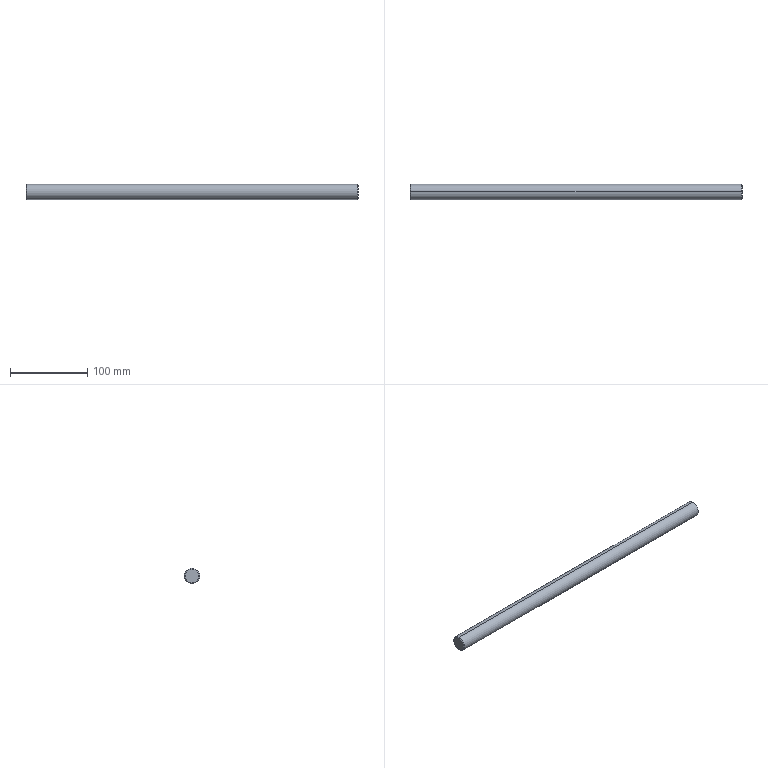Part | STEP file | 001-006-SAD21_D20_L430 | 1 solid | 8 faces | box 430 x 20 x 20 mm | volume 135028 mm3 | cone 4 | cylinder 2 | plane 2 | commonest cylinder face diameters 20 x2
STEP:
#1=CARTESIAN_POINT('',(0.,0.,0.));
#2=DIRECTION('',(0.,0.,1.));
#3=DIRECTION('',(1.,0.,0.));
#4=AXIS2_PLACEMENT_3D('',#1,#2,#3);
#5=CARTESIAN_POINT('',(430.,0.,9.));
#6=VERTEX_POINT('',#5);
#7=CARTESIAN_POINT('',(430.,0.,-9.));
#8=VERTEX_POINT('',#7);
#9=CARTESIAN_POINT('',(430.,0.,0.));
#10=DIRECTION('',(-1.,0.,0.));
#11=DIRECTION('',(0.,0.,1.));
#12=AXIS2_PLACEMENT_3D('',#9,#10,#11);
#13=CIRCLE('',#12,9.);
#14=CARTESIAN_POINT('',(430.,0.,0.));
#15=DIRECTION('',(-1.,0.,0.));
#16=DIRECTION('',(0.,0.,1.));
#17=AXIS2_PLACEMENT_3D('',#14,#15,#16);
#18=CONICAL_SURFACE('',#17,9.,0.7854);
#19=CARTESIAN_POINT('',(0.,0.));
#20=DIRECTION('',(1.,0.));
#21=VECTOR('',#20,1.);
#22=LINE('',#19,#21);
#23=(GEOMETRIC_REPRESENTATION_CONTEXT(2)PARAMETRIC_REPRESENTATION_CONTEXT()REPRESENTATION_CONTEXT('',''));
#24=DEFINITIONAL_REPRESENTATION('',(#22),#23);
#25=PCURVE('',#18,#24);
#26=CARTESIAN_POINT('',(430.,9.,0.));
#27=DIRECTION('',(-1.,0.,0.));
#28=DIRECTION('',(0.,0.,1.));
#29=AXIS2_PLACEMENT_3D('',#26,#27,#28);
#30=PLANE('',#29);
#31=CARTESIAN_POINT('',(0.,-9.));
#32=DIRECTION('',(1.,0.));
#33=AXIS2_PLACEMENT_2D('',#31,#32);
#34=CIRCLE('',#33,9.);
#35=(GEOMETRIC_REPRESENTATION_CONTEXT(2)PARAMETRIC_REPRESENTATION_CONTEXT()REPRESENTATION_CONTEXT('',''));
#36=DEFINITIONAL_REPRESENTATION('',(#34),#35);
#37=PCURVE('',#30,#36);
#38=SURFACE_CURVE('',#13,(#25,#37),.PCURVE_S1.);
#39=EDGE_CURVE('',#6,#8,#38,.T.);
#40=ORIENTED_EDGE('',*,*,#39,.T.);
#41=CARTESIAN_POINT('',(429.,0.,-10.));
#42=VERTEX_POINT('',#41);
#43=CARTESIAN_POINT('',(430.,0.,-9.));
#44=DIRECTION('',(-0.7071,0.,-0.7071));
#45=VECTOR('',#44,1.);
#46=LINE('',#43,#45);
#47=CARTESIAN_POINT('',(3.142,0.));
#48=DIRECTION('',(0.,1.));
#49=VECTOR('',#48,1.);
#50=LINE('',#47,#49);
#51=(GEOMETRIC_REPRESENTATION_CONTEXT(2)PARAMETRIC_REPRESENTATION_CONTEXT()REPRESENTATION_CONTEXT('',''));
#52=DEFINITIONAL_REPRESENTATION('',(#50),#51);
#53=PCURVE('',#18,#52);
#54=CARTESIAN_POINT('',(430.,0.,0.));
#55=DIRECTION('',(-1.,0.,0.));
#56=DIRECTION('',(0.,0.,1.));
#57=AXIS2_PLACEMENT_3D('',#54,#55,#56);
#58=CONICAL_SURFACE('',#57,9.,0.7854);
#59=CARTESIAN_POINT('',(3.142,0.));
#60=DIRECTION('',(0.,1.));
#61=VECTOR('',#60,1.);
#62=LINE('',#59,#61);
#63=(GEOMETRIC_REPRESENTATION_CONTEXT(2)PARAMETRIC_REPRESENTATION_CONTEXT()REPRESENTATION_CONTEXT('',''));
#64=DEFINITIONAL_REPRESENTATION('',(#62),#63);
#65=PCURVE('',#58,#64);
#66=SURFACE_CURVE('',#46,(#53,#65),.PCURVE_S1.);
#67=EDGE_CURVE('',#8,#42,#66,.T.);
#68=ORIENTED_EDGE('',*,*,#67,.T.);
#69=CARTESIAN_POINT('',(429.,0.,10.));
#70=VERTEX_POINT('',#69);
#71=CARTESIAN_POINT('',(429.,0.,0.));
#72=DIRECTION('',(-1.,0.,0.));
#73=DIRECTION('',(0.,0.,1.));
#74=AXIS2_PLACEMENT_3D('',#71,#72,#73);
#75=CIRCLE('',#74,10.);
#76=CARTESIAN_POINT('',(0.,1.));
#77=DIRECTION('',(1.,0.));
#78=VECTOR('',#77,1.);
#79=LINE('',#76,#78);
#80=(GEOMETRIC_REPRESENTATION_CONTEXT(2)PARAMETRIC_REPRESENTATION_CONTEXT()REPRESENTATION_CONTEXT('',''));
#81=DEFINITIONAL_REPRESENTATION('',(#79),#80);
#82=PCURVE('',#18,#81);
#83=CARTESIAN_POINT('',(430.,0.,0.));
#84=DIRECTION('',(-1.,0.,0.));
#85=DIRECTION('',(0.,0.,1.));
#86=AXIS2_PLACEMENT_3D('',#83,#84,#85);
#87=CYLINDRICAL_SURFACE('',#86,10.);
#88=CARTESIAN_POINT('',(0.,1.));
#89=DIRECTION('',(1.,0.));
#90=VECTOR('',#89,1.);
#91=LINE('',#88,#90);
#92=(GEOMETRIC_REPRESENTATION_CONTEXT(2)PARAMETRIC_REPRESENTATION_CONTEXT()REPRESENTATION_CONTEXT('',''));
#93=DEFINITIONAL_REPRESENTATION('',(#91),#92);
#94=PCURVE('',#87,#93);
#95=SURFACE_CURVE('',#75,(#82,#94),.PCURVE_S1.);
#96=EDGE_CURVE('',#70,#42,#95,.T.);
#97=ORIENTED_EDGE('',*,*,#96,.F.);
#98=CARTESIAN_POINT('',(430.,0.,9.));
#99=DIRECTION('',(-0.7071,0.,0.7071));
#100=VECTOR('',#99,1.);
#101=LINE('',#98,#100);
#102=CARTESIAN_POINT('',(0.,0.));
#103=DIRECTION('',(0.,1.));
#104=VECTOR('',#103,1.);
#105=LINE('',#102,#104);
#106=(GEOMETRIC_REPRESENTATION_CONTEXT(2)PARAMETRIC_REPRESENTATION_CONTEXT()REPRESENTATION_CONTEXT('',''));
#107=DEFINITIONAL_REPRESENTATION('',(#105),#106);
#108=PCURVE('',#18,#107);
#109=CARTESIAN_POINT('',(6.283,0.));
#110=DIRECTION('',(0.,1.));
#111=VECTOR('',#110,1.);
#112=LINE('',#109,#111);
#113=(GEOMETRIC_REPRESENTATION_CONTEXT(2)PARAMETRIC_REPRESENTATION_CONTEXT()REPRESENTATION_CONTEXT('',''));
#114=DEFINITIONAL_REPRESENTATION('',(#112),#113);
#115=PCURVE('',#58,#114);
#116=SURFACE_CURVE('',#101,(#108,#115),.PCURVE_S1.);
#117=EDGE_CURVE('',#6,#70,#116,.T.);
#118=ORIENTED_EDGE('',*,*,#117,.F.);
#119=EDGE_LOOP('',(#40,#68,#97,#118));
#120=FACE_BOUND('',#119,.T.);
#121=ADVANCED_FACE('',(#120),#18,.T.);
#122=ORIENTED_EDGE('',*,*,#96,.T.);
#123=CARTESIAN_POINT('',(1.,0.,-10.));
#124=VERTEX_POINT('',#123);
#125=CARTESIAN_POINT('',(430.,0.,-10.));
#126=DIRECTION('',(-1.,0.,0.));
#127=VECTOR('',#126,1.);
#128=LINE('',#125,#127);
#129=CARTESIAN_POINT('',(3.142,0.));
#130=DIRECTION('',(0.,1.));
#131=VECTOR('',#130,1.);
#132=LINE('',#129,#131);
#133=(GEOMETRIC_REPRESENTATION_CONTEXT(2)PARAMETRIC_REPRESENTATION_CONTEXT()REPRESENTATION_CONTEXT('',''));
#134=DEFINITIONAL_REPRESENTATION('',(#132),#133);
#135=PCURVE('',#87,#134);
#136=CARTESIAN_POINT('',(430.,0.,0.));
#137=DIRECTION('',(-1.,0.,0.));
#138=DIRECTION('',(0.,0.,1.));
#139=AXIS2_PLACEMENT_3D('',#136,#137,#138);
#140=CYLINDRICAL_SURFACE('',#139,10.);
#141=CARTESIAN_POINT('',(3.142,0.));
#142=DIRECTION('',(0.,1.));
#143=VECTOR('',#142,1.);
#144=LINE('',#141,#143);
#145=(GEOMETRIC_REPRESENTATION_CONTEXT(2)PARAMETRIC_REPRESENTATION_CONTEXT()REPRESENTATION_CONTEXT('',''));
#146=DEFINITIONAL_REPRESENTATION('',(#144),#145);
#147=PCURVE('',#140,#146);
#148=SURFACE_CURVE('',#128,(#135,#147),.PCURVE_S1.);
#149=EDGE_CURVE('',#42,#124,#148,.T.);
#150=ORIENTED_EDGE('',*,*,#149,.T.);
#151=CARTESIAN_POINT('',(1.,0.,10.));
#152=VERTEX_POINT('',#151);
#153=CARTESIAN_POINT('',(1.,0.,0.));
#154=DIRECTION('',(-1.,0.,0.));
#155=DIRECTION('',(0.,0.,1.));
#156=AXIS2_PLACEMENT_3D('',#153,#154,#155);
#157=CIRCLE('',#156,10.);
#158=CARTESIAN_POINT('',(0.,429.));
#159=DIRECTION('',(1.,0.));
#160=VECTOR('',#159,1.);
#161=LINE('',#158,#160);
#162=(GEOMETRIC_REPRESENTATION_CONTEXT(2)PARAMETRIC_REPRESENTATION_CONTEXT()REPRESENTATION_CONTEXT('',''));
#163=DEFINITIONAL_REPRESENTATION('',(#161),#162);
#164=PCURVE('',#87,#163);
#165=CARTESIAN_POINT('',(1.,0.,0.));
#166=DIRECTION('',(1.,0.,0.));
#167=DIRECTION('',(0.,0.,-1.));
#168=AXIS2_PLACEMENT_3D('',#165,#166,#167);
#169=CONICAL_SURFACE('',#168,10.,0.7854);
#170=CARTESIAN_POINT('',(3.142,0.));
#171=DIRECTION('',(-1.,0.));
#172=VECTOR('',#171,1.);
#173=LINE('',#170,#172);
#174=(GEOMETRIC_REPRESENTATION_CONTEXT(2)PARAMETRIC_REPRESENTATION_CONTEXT()REPRESENTATION_CONTEXT('',''));
#175=DEFINITIONAL_REPRESENTATION('',(#173),#174);
#176=PCURVE('',#169,#175);
#177=SURFACE_CURVE('',#157,(#164,#176),.PCURVE_S1.);
#178=EDGE_CURVE('',#152,#124,#177,.T.);
#179=ORIENTED_EDGE('',*,*,#178,.F.);
#180=CARTESIAN_POINT('',(430.,0.,10.));
#181=DIRECTION('',(-1.,0.,0.));
#182=VECTOR('',#181,1.);
#183=LINE('',#180,#182);
#184=CARTESIAN_POINT('',(0.,0.));
#185=DIRECTION('',(0.,1.));
#186=VECTOR('',#185,1.);
#187=LINE('',#184,#186);
#188=(GEOMETRIC_REPRESENTATION_CONTEXT(2)PARAMETRIC_REPRESENTATION_CONTEXT()REPRESENTATION_CONTEXT('',''));
#189=DEFINITIONAL_REPRESENTATION('',(#187),#188);
#190=PCURVE('',#87,#189);
#191=CARTESIAN_POINT('',(6.283,0.));
#192=DIRECTION('',(0.,1.));
#193=VECTOR('',#192,1.);
#194=LINE('',#191,#193);
#195=(GEOMETRIC_REPRESENTATION_CONTEXT(2)PARAMETRIC_REPRESENTATION_CONTEXT()REPRESENTATION_CONTEXT('',''));
#196=DEFINITIONAL_REPRESENTATION('',(#194),#195);
#197=PCURVE('',#140,#196);
#198=SURFACE_CURVE('',#183,(#190,#197),.PCURVE_S1.);
#199=EDGE_CURVE('',#70,#152,#198,.T.);
#200=ORIENTED_EDGE('',*,*,#199,.F.);
#201=EDGE_LOOP('',(#122,#150,#179,#200));
#202=FACE_BOUND('',#201,.T.);
#203=ADVANCED_FACE('',(#202),#87,.T.);
#204=CARTESIAN_POINT('',(0.,0.,9.));
#205=VERTEX_POINT('',#204);
#206=CARTESIAN_POINT('',(0.,0.,-9.));
#207=VERTEX_POINT('',#206);
#208=CARTESIAN_POINT('',(0.,0.,0.));
#209=DIRECTION('',(-1.,0.,0.));
#210=DIRECTION('',(0.,0.,1.));
#211=AXIS2_PLACEMENT_3D('',#208,#209,#210);
#212=CIRCLE('',#211,9.);
#213=CARTESIAN_POINT('',(3.142,-1.));
#214=DIRECTION('',(-1.,0.));
#215=VECTOR('',#214,1.);
#216=LINE('',#213,#215);
#217=(GEOMETRIC_REPRESENTATION_CONTEXT(2)PARAMETRIC_REPRESENTATION_CONTEXT()REPRESENTATION_CONTEXT('',''));
#218=DEFINITIONAL_REPRESENTATION('',(#216),#217);
#219=PCURVE('',#169,#218);
#220=CARTESIAN_POINT('',(0.,0.,0.));
#221=DIRECTION('',(1.,0.,0.));
#222=DIRECTION('',(0.,0.,-1.));
#223=AXIS2_PLACEMENT_3D('',#220,#221,#222);
#224=PLANE('',#223);
#225=CARTESIAN_POINT('',(-9.,0.));
#226=CARTESIAN_POINT('',(-9.,15.588));
#227=CARTESIAN_POINT('',(4.5,7.794));
#228=CARTESIAN_POINT('',(18.,0.));
#229=CARTESIAN_POINT('',(4.5,-7.794));
#230=CARTESIAN_POINT('',(-9.,-15.588));
#231=CARTESIAN_POINT('',(-9.,0.));
#232=(BOUNDED_CURVE()B_SPLINE_CURVE(2,(#225,#226,#227,#228,#229,#230,#231),.UNSPECIFIED.,.T.,.F.)B_SPLINE_CURVE_WITH_KNOTS((1,2,2,2,2,1),(-2.094,0.,2.094,4.189,6.283,8.378),.UNSPECIFIED.)CURVE()GEOMETRIC_REPRESENTATION_ITEM()RATIONAL_B_SPLINE_CURVE((1.,0.5,1.,0.5,1.,0.5,1.))REPRESENTATION_ITEM(''));
#233=(GEOMETRIC_REPRESENTATION_CONTEXT(2)PARAMETRIC_REPRESENTATION_CONTEXT()REPRESENTATION_CONTEXT('',''));
#234=DEFINITIONAL_REPRESENTATION('',(#232),#233);
#235=PCURVE('',#224,#234);
#236=SURFACE_CURVE('',#212,(#219,#235),.PCURVE_S1.);
#237=EDGE_CURVE('',#205,#207,#236,.T.);
#238=ORIENTED_EDGE('',*,*,#237,.F.);
#239=CARTESIAN_POINT('',(1.,0.,10.));
#240=DIRECTION('',(0.7071,0.,0.7071));
#241=VECTOR('',#240,1.);
#242=LINE('',#239,#241);
#243=CARTESIAN_POINT('',(3.142,0.));
#244=DIRECTION('',(0.,1.));
#245=VECTOR('',#244,1.);
#246=LINE('',#243,#245);
#247=(GEOMETRIC_REPRESENTATION_CONTEXT(2)PARAMETRIC_REPRESENTATION_CONTEXT()REPRESENTATION_CONTEXT('',''));
#248=DEFINITIONAL_REPRESENTATION('',(#246),#247);
#249=PCURVE('',#169,#248);
#250=CARTESIAN_POINT('',(1.,0.,0.));
#251=DIRECTION('',(1.,0.,0.));
#252=DIRECTION('',(0.,0.,-1.));
#253=AXIS2_PLACEMENT_3D('',#250,#251,#252);
#254=CONICAL_SURFACE('',#253,10.,0.7854);
#255=CARTESIAN_POINT('',(3.142,0.));
#256=DIRECTION('',(0.,1.));
#257=VECTOR('',#256,1.);
#258=LINE('',#255,#257);
#259=(GEOMETRIC_REPRESENTATION_CONTEXT(2)PARAMETRIC_REPRESENTATION_CONTEXT()REPRESENTATION_CONTEXT('',''));
#260=DEFINITIONAL_REPRESENTATION('',(#258),#259);
#261=PCURVE('',#254,#260);
#262=SURFACE_CURVE('',#242,(#249,#261),.PCURVE_S1.);
#263=EDGE_CURVE('',#205,#152,#262,.T.);
#264=ORIENTED_EDGE('',*,*,#263,.T.);
#265=ORIENTED_EDGE('',*,*,#178,.T.);
#266=CARTESIAN_POINT('',(1.,0.,-10.));
#267=DIRECTION('',(0.7071,0.,-0.7071));
#268=VECTOR('',#267,1.);
#269=LINE('',#266,#268);
#270=CARTESIAN_POINT('',(0.,0.));
#271=DIRECTION('',(0.,1.));
#272=VECTOR('',#271,1.);
#273=LINE('',#270,#272);
#274=(GEOMETRIC_REPRESENTATION_CONTEXT(2)PARAMETRIC_REPRESENTATION_CONTEXT()REPRESENTATION_CONTEXT('',''));
#275=DEFINITIONAL_REPRESENTATION('',(#273),#274);
#276=PCURVE('',#169,#275);
#277=CARTESIAN_POINT('',(6.283,0.));
#278=DIRECTION('',(0.,1.));
#279=VECTOR('',#278,1.);
#280=LINE('',#277,#279);
#281=(GEOMETRIC_REPRESENTATION_CONTEXT(2)PARAMETRIC_REPRESENTATION_CONTEXT()REPRESENTATION_CONTEXT('',''));
#282=DEFINITIONAL_REPRESENTATION('',(#280),#281);
#283=PCURVE('',#254,#282);
#284=SURFACE_CURVE('',#269,(#276,#283),.PCURVE_S1.);
#285=EDGE_CURVE('',#207,#124,#284,.T.);
#286=ORIENTED_EDGE('',*,*,#285,.F.);
#287=EDGE_LOOP('',(#238,#264,#265,#286));
#288=FACE_BOUND('',#287,.T.);
#289=ADVANCED_FACE('',(#288),#169,.T.);
#290=CARTESIAN_POINT('',(0.,0.,0.));
#291=DIRECTION('',(-1.,0.,0.));
#292=DIRECTION('',(0.,0.,1.));
#293=AXIS2_PLACEMENT_3D('',#290,#291,#292);
#294=CIRCLE('',#293,9.);
#295=CARTESIAN_POINT('',(-9.,0.));
#296=CARTESIAN_POINT('',(-9.,15.588));
#297=CARTESIAN_POINT('',(4.5,7.794));
#298=CARTESIAN_POINT('',(18.,0.));
#299=CARTESIAN_POINT('',(4.5,-7.794));
#300=CARTESIAN_POINT('',(-9.,-15.588));
#301=CARTESIAN_POINT('',(-9.,0.));
#302=(BOUNDED_CURVE()B_SPLINE_CURVE(2,(#295,#296,#297,#298,#299,#300,#301),.UNSPECIFIED.,.T.,.F.)B_SPLINE_CURVE_WITH_KNOTS((1,2,2,2,2,1),(-2.094,0.,2.094,4.189,6.283,8.378),.UNSPECIFIED.)CURVE()GEOMETRIC_REPRESENTATION_ITEM()RATIONAL_B_SPLINE_CURVE((1.,0.5,1.,0.5,1.,0.5,1.))REPRESENTATION_ITEM(''));
#303=(GEOMETRIC_REPRESENTATION_CONTEXT(2)PARAMETRIC_REPRESENTATION_CONTEXT()REPRESENTATION_CONTEXT('',''));
#304=DEFINITIONAL_REPRESENTATION('',(#302),#303);
#305=PCURVE('',#224,#304);
#306=CARTESIAN_POINT('',(9.425,-1.));
#307=DIRECTION('',(-1.,0.));
#308=VECTOR('',#307,1.);
#309=LINE('',#306,#308);
#310=(GEOMETRIC_REPRESENTATION_CONTEXT(2)PARAMETRIC_REPRESENTATION_CONTEXT()REPRESENTATION_CONTEXT('',''));
#311=DEFINITIONAL_REPRESENTATION('',(#309),#310);
#312=PCURVE('',#254,#311);
#313=SURFACE_CURVE('',#294,(#305,#312),.PCURVE_S1.);
#314=EDGE_CURVE('',#207,#205,#313,.T.);
#315=ORIENTED_EDGE('',*,*,#314,.T.);
#316=ORIENTED_EDGE('',*,*,#237,.T.);
#317=EDGE_LOOP('',(#315,#316));
#318=FACE_BOUND('',#317,.T.);
#319=ADVANCED_FACE('',(#318),#224,.F.);
#320=ORIENTED_EDGE('',*,*,#263,.F.);
#321=ORIENTED_EDGE('',*,*,#314,.F.);
#322=ORIENTED_EDGE('',*,*,#285,.T.);
#323=CARTESIAN_POINT('',(1.,0.,0.));
#324=DIRECTION('',(-1.,0.,0.));
#325=DIRECTION('',(0.,0.,1.));
#326=AXIS2_PLACEMENT_3D('',#323,#324,#325);
#327=CIRCLE('',#326,10.);
#328=CARTESIAN_POINT('',(9.425,0.));
#329=DIRECTION('',(-1.,0.));
#330=VECTOR('',#329,1.);
#331=LINE('',#328,#330);
#332=(GEOMETRIC_REPRESENTATION_CONTEXT(2)PARAMETRIC_REPRESENTATION_CONTEXT()REPRESENTATION_CONTEXT('',''));
#333=DEFINITIONAL_REPRESENTATION('',(#331),#332);
#334=PCURVE('',#254,#333);
#335=CARTESIAN_POINT('',(0.,429.));
#336=DIRECTION('',(1.,0.));
#337=VECTOR('',#336,1.);
#338=LINE('',#335,#337);
#339=(GEOMETRIC_REPRESENTATION_CONTEXT(2)PARAMETRIC_REPRESENTATION_CONTEXT()REPRESENTATION_CONTEXT('',''));
#340=DEFINITIONAL_REPRESENTATION('',(#338),#339);
#341=PCURVE('',#140,#340);
#342=SURFACE_CURVE('',#327,(#334,#341),.PCURVE_S1.);
#343=EDGE_CURVE('',#124,#152,#342,.T.);
#344=ORIENTED_EDGE('',*,*,#343,.T.);
#345=EDGE_LOOP('',(#320,#321,#322,#344));
#346=FACE_BOUND('',#345,.T.);
#347=ADVANCED_FACE('',(#346),#254,.T.);
#348=ORIENTED_EDGE('',*,*,#149,.F.);
#349=CARTESIAN_POINT('',(429.,0.,0.));
#350=DIRECTION('',(-1.,0.,0.));
#351=DIRECTION('',(0.,0.,1.));
#352=AXIS2_PLACEMENT_3D('',#349,#350,#351);
#353=CIRCLE('',#352,10.);
#354=CARTESIAN_POINT('',(0.,1.));
#355=DIRECTION('',(1.,0.));
#356=VECTOR('',#355,1.);
#357=LINE('',#354,#356);
#358=(GEOMETRIC_REPRESENTATION_CONTEXT(2)PARAMETRIC_REPRESENTATION_CONTEXT()REPRESENTATION_CONTEXT('',''));
#359=DEFINITIONAL_REPRESENTATION('',(#357),#358);
#360=PCURVE('',#140,#359);
#361=CARTESIAN_POINT('',(0.,1.));
#362=DIRECTION('',(1.,0.));
#363=VECTOR('',#362,1.);
#364=LINE('',#361,#363);
#365=(GEOMETRIC_REPRESENTATION_CONTEXT(2)PARAMETRIC_REPRESENTATION_CONTEXT()REPRESENTATION_CONTEXT('',''));
#366=DEFINITIONAL_REPRESENTATION('',(#364),#365);
#367=PCURVE('',#58,#366);
#368=SURFACE_CURVE('',#353,(#360,#367),.PCURVE_S1.);
#369=EDGE_CURVE('',#42,#70,#368,.T.);
#370=ORIENTED_EDGE('',*,*,#369,.T.);
#371=ORIENTED_EDGE('',*,*,#199,.T.);
#372=ORIENTED_EDGE('',*,*,#343,.F.);
#373=EDGE_LOOP('',(#348,#370,#371,#372));
#374=FACE_BOUND('',#373,.T.);
#375=ADVANCED_FACE('',(#374),#140,.T.);
#376=ORIENTED_EDGE('',*,*,#67,.F.);
#377=CARTESIAN_POINT('',(430.,0.,0.));
#378=DIRECTION('',(-1.,0.,0.));
#379=DIRECTION('',(0.,0.,1.));
#380=AXIS2_PLACEMENT_3D('',#377,#378,#379);
#381=CIRCLE('',#380,9.);
#382=CARTESIAN_POINT('',(0.,0.));
#383=DIRECTION('',(1.,0.));
#384=VECTOR('',#383,1.);
#385=LINE('',#382,#384);
#386=(GEOMETRIC_REPRESENTATION_CONTEXT(2)PARAMETRIC_REPRESENTATION_CONTEXT()REPRESENTATION_CONTEXT('',''));
#387=DEFINITIONAL_REPRESENTATION('',(#385),#386);
#388=PCURVE('',#58,#387);
#389=CARTESIAN_POINT('',(0.,-9.));
#390=DIRECTION('',(1.,0.));
#391=AXIS2_PLACEMENT_2D('',#389,#390);
#392=CIRCLE('',#391,9.);
#393=(GEOMETRIC_REPRESENTATION_CONTEXT(2)PARAMETRIC_REPRESENTATION_CONTEXT()REPRESENTATION_CONTEXT('',''));
#394=DEFINITIONAL_REPRESENTATION('',(#392),#393);
#395=PCURVE('',#30,#394);
#396=SURFACE_CURVE('',#381,(#388,#395),.PCURVE_S1.);
#397=EDGE_CURVE('',#8,#6,#396,.T.);
#398=ORIENTED_EDGE('',*,*,#397,.T.);
#399=ORIENTED_EDGE('',*,*,#117,.T.);
#400=ORIENTED_EDGE('',*,*,#369,.F.);
#401=EDGE_LOOP('',(#376,#398,#399,#400));
#402=FACE_BOUND('',#401,.T.);
#403=ADVANCED_FACE('',(#402),#58,.T.);
#404=ORIENTED_EDGE('',*,*,#39,.F.);
#405=ORIENTED_EDGE('',*,*,#397,.F.);
#406=EDGE_LOOP('',(#404,#405));
#407=FACE_BOUND('',#406,.T.);
#408=ADVANCED_FACE('',(#407),#30,.F.);
#409=CLOSED_SHELL('',(#121,#203,#289,#319,#347,#375,#403,#408));
#410=MANIFOLD_SOLID_BREP('',#409);
#411=(LENGTH_UNIT()NAMED_UNIT(*)SI_UNIT(.MILLI.,.METRE.));
#412=UNCERTAINTY_MEASURE_WITH_UNIT(LENGTH_MEASURE(0.0000001),#411,'','');
#413=(NAMED_UNIT(*)PLANE_ANGLE_UNIT()SI_UNIT($,.RADIAN.));
#414=(NAMED_UNIT(*)SI_UNIT($,.STERADIAN.)SOLID_ANGLE_UNIT());
#415=(GEOMETRIC_REPRESENTATION_CONTEXT(3)GLOBAL_UNCERTAINTY_ASSIGNED_CONTEXT((#412))GLOBAL_UNIT_ASSIGNED_CONTEXT((#411,#413,#414))REPRESENTATION_CONTEXT('',''));
#416=ADVANCED_BREP_SHAPE_REPRESENTATION('',(#4,#410),#415);